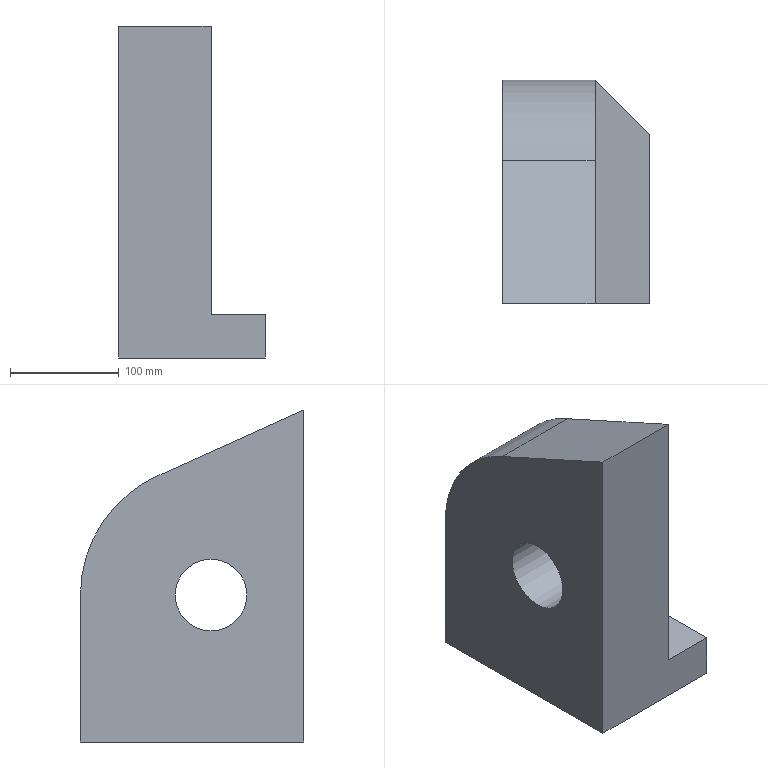Part | NX | features solid 2 | 1 solid | 11 faces | box 135 x 205 x 305 mm | volume 4488992 mm3 | plane 9 | cylinder 2 | commonest cylinder face diameters 66 x1 240 x1
STEP:
#1=CARTESIAN_POINT('',(1415.,1020.,-375.));
#2=VERTEX_POINT('',#1);
#3=CARTESIAN_POINT('',(1415.,1020.,-680.));
#4=VERTEX_POINT('',#3);
#5=CARTESIAN_POINT('',(1415.,1020.,-330.));
#6=DIRECTION('',(0.,0.,-1.));
#7=VECTOR('',#6,1000.);
#8=LINE('',#5,#7);
#9=EDGE_CURVE('',#2,#4,#8,.T.);
#10=ORIENTED_EDGE('',*,*,#9,.T.);
#11=CARTESIAN_POINT('',(1550.,1020.,-680.));
#12=VERTEX_POINT('',#11);
#13=CARTESIAN_POINT('',(1550.,1020.,-680.));
#14=DIRECTION('',(1.,0.,0.));
#15=VECTOR('',#14,1000.);
#16=LINE('',#13,#15);
#17=EDGE_CURVE('',#4,#12,#16,.T.);
#18=ORIENTED_EDGE('',*,*,#17,.T.);
#19=CARTESIAN_POINT('',(1550.,1020.,-640.));
#20=VERTEX_POINT('',#19);
#21=CARTESIAN_POINT('',(1550.,1020.,-575.));
#22=DIRECTION('',(0.,0.,1.));
#23=VECTOR('',#22,1000.);
#24=LINE('',#21,#23);
#25=EDGE_CURVE('',#12,#20,#24,.T.);
#26=ORIENTED_EDGE('',*,*,#25,.T.);
#27=CARTESIAN_POINT('',(1500.,1020.,-640.));
#28=VERTEX_POINT('',#27);
#29=CARTESIAN_POINT('',(-1361.187,1020.,-640.));
#30=DIRECTION('',(1.,0.,0.));
#31=VECTOR('',#30,1000.);
#32=LINE('',#29,#31);
#33=EDGE_CURVE('',#28,#20,#32,.T.);
#34=ORIENTED_EDGE('',*,*,#33,.F.);
#35=CARTESIAN_POINT('',(1500.,1020.,-375.));
#36=VERTEX_POINT('',#35);
#37=CARTESIAN_POINT('',(1500.,1020.,-330.));
#38=DIRECTION('',(0.,0.,-1.));
#39=VECTOR('',#38,1000.);
#40=LINE('',#37,#39);
#41=EDGE_CURVE('',#36,#28,#40,.T.);
#42=ORIENTED_EDGE('',*,*,#41,.F.);
#43=CARTESIAN_POINT('',(1550.,1020.,-375.));
#44=DIRECTION('',(1.,0.,0.));
#45=VECTOR('',#44,1000.);
#46=LINE('',#43,#45);
#47=EDGE_CURVE('',#2,#36,#46,.T.);
#48=ORIENTED_EDGE('',*,*,#47,.F.);
#49=EDGE_LOOP('',(#10,#18,#26,#34,#42,#48));
#50=FACE_BOUND('',#49,.T.);
#51=CARTESIAN_POINT('',(1550.,1020.,-425.));
#52=DIRECTION('',(0.,-1.,0.));
#53=DIRECTION('',(0.,0.,1.));
#54=AXIS2_PLACEMENT_3D('',#51,#52,#53);
#55=PLANE('',#54);
#56=ADVANCED_FACE('',(#50),#55,.T.);
#57=ORIENTED_EDGE('',*,*,#25,.F.);
#58=CARTESIAN_POINT('',(1550.,1175.,-680.));
#59=VERTEX_POINT('',#58);
#60=CARTESIAN_POINT('',(1550.,-830.,-680.));
#61=DIRECTION('',(0.,1.,0.));
#62=VECTOR('',#61,1000.);
#63=LINE('',#60,#62);
#64=EDGE_CURVE('',#12,#59,#63,.T.);
#65=ORIENTED_EDGE('',*,*,#64,.T.);
#66=CARTESIAN_POINT('',(1550.,1175.,-640.));
#67=VERTEX_POINT('',#66);
#68=CARTESIAN_POINT('',(1550.,1175.,-615.));
#69=DIRECTION('',(0.,0.,-1.));
#70=VECTOR('',#69,1000.);
#71=LINE('',#68,#70);
#72=EDGE_CURVE('',#59,#67,#71,.F.);
#73=ORIENTED_EDGE('',*,*,#72,.T.);
#74=CARTESIAN_POINT('',(1550.,-830.,-640.));
#75=DIRECTION('',(0.,-1.,0.));
#76=VECTOR('',#75,1000.);
#77=LINE('',#74,#76);
#78=EDGE_CURVE('',#67,#20,#77,.T.);
#79=ORIENTED_EDGE('',*,*,#78,.T.);
#80=EDGE_LOOP('',(#57,#65,#73,#79));
#81=FACE_BOUND('',#80,.T.);
#82=CARTESIAN_POINT('',(1550.,-830.,-575.));
#83=DIRECTION('',(1.,0.,0.));
#84=DIRECTION('',(0.,0.,1.));
#85=AXIS2_PLACEMENT_3D('',#82,#83,#84);
#86=PLANE('',#85);
#87=ADVANCED_FACE('',(#81),#86,.T.);
#88=ORIENTED_EDGE('',*,*,#33,.T.);
#89=ORIENTED_EDGE('',*,*,#78,.F.);
#90=CARTESIAN_POINT('',(1500.,1225.,-640.));
#91=VERTEX_POINT('',#90);
#92=CARTESIAN_POINT('',(171.907,2553.093,-640.));
#93=DIRECTION('',(0.7071,-0.7071,0.));
#94=VECTOR('',#93,1000.);
#95=LINE('',#92,#94);
#96=EDGE_CURVE('',#67,#91,#95,.F.);
#97=ORIENTED_EDGE('',*,*,#96,.T.);
#98=CARTESIAN_POINT('',(1500.,1230.,-640.));
#99=DIRECTION('',(0.,-1.,0.));
#100=VECTOR('',#99,1000.);
#101=LINE('',#98,#100);
#102=EDGE_CURVE('',#91,#28,#101,.T.);
#103=ORIENTED_EDGE('',*,*,#102,.T.);
#104=EDGE_LOOP('',(#88,#89,#97,#103));
#105=FACE_BOUND('',#104,.T.);
#106=CARTESIAN_POINT('',(-1361.187,1020.,-640.));
#107=DIRECTION('',(0.,0.,-1.));
#108=DIRECTION('',(-1.,0.,0.));
#109=AXIS2_PLACEMENT_3D('',#106,#107,#108);
#110=PLANE('',#109);
#111=ADVANCED_FACE('',(#105),#110,.F.);
#112=CARTESIAN_POINT('',(1500.,1150.971,-434.155));
#113=VERTEX_POINT('',#112);
#114=CARTESIAN_POINT('',(1500.,1177.538,-446.154));
#115=DIRECTION('',(0.,0.9114,-0.4116));
#116=VECTOR('',#115,1000.);
#117=LINE('',#114,#116);
#118=EDGE_CURVE('',#36,#113,#117,.T.);
#119=ORIENTED_EDGE('',*,*,#118,.F.);
#120=ORIENTED_EDGE('',*,*,#41,.T.);
#121=ORIENTED_EDGE('',*,*,#102,.F.);
#122=CARTESIAN_POINT('',(1500.,1225.,-545.));
#123=VERTEX_POINT('',#122);
#124=CARTESIAN_POINT('',(1500.,1225.,-560.));
#125=DIRECTION('',(0.,0.,-1.));
#126=VECTOR('',#125,1000.);
#127=LINE('',#124,#126);
#128=EDGE_CURVE('',#123,#91,#127,.T.);
#129=ORIENTED_EDGE('',*,*,#128,.F.);
#130=CARTESIAN_POINT('',(1500.,1105.,-545.));
#131=DIRECTION('',(-1.,0.,0.));
#132=DIRECTION('',(0.,0.,-1.));
#133=AXIS2_PLACEMENT_3D('',#130,#131,#132);
#134=CIRCLE('',#133,120.);
#135=EDGE_CURVE('',#123,#113,#134,.F.);
#136=ORIENTED_EDGE('',*,*,#135,.T.);
#137=EDGE_LOOP('',(#119,#120,#121,#129,#136));
#138=FACE_BOUND('',#137,.T.);
#139=CARTESIAN_POINT('',(1500.,1105.,-578.));
#140=VERTEX_POINT('',#139);
#141=CARTESIAN_POINT('',(1500.,1105.,-545.));
#142=DIRECTION('',(-1.,0.,0.));
#143=DIRECTION('',(0.,0.,-1.));
#144=AXIS2_PLACEMENT_3D('',#141,#142,#143);
#145=CIRCLE('',#144,33.);
#146=EDGE_CURVE('',#140,#140,#145,.T.);
#147=ORIENTED_EDGE('',*,*,#146,.T.);
#148=EDGE_LOOP('',(#147));
#149=FACE_BOUND('',#148,.T.);
#150=CARTESIAN_POINT('',(1500.,1230.,-330.));
#151=DIRECTION('',(1.,0.,0.));
#152=DIRECTION('',(0.,1.,0.));
#153=AXIS2_PLACEMENT_3D('',#150,#151,#152);
#154=PLANE('',#153);
#155=ADVANCED_FACE('',(#138,#149),#154,.T.);
#156=ORIENTED_EDGE('',*,*,#146,.F.);
#157=EDGE_LOOP('',(#156));
#158=FACE_BOUND('',#157,.T.);
#159=CARTESIAN_POINT('',(1415.,1105.,-578.));
#160=VERTEX_POINT('',#159);
#161=CARTESIAN_POINT('',(1415.,1105.,-545.));
#162=DIRECTION('',(-1.,0.,0.));
#163=DIRECTION('',(0.,0.,-1.));
#164=AXIS2_PLACEMENT_3D('',#161,#162,#163);
#165=CIRCLE('',#164,33.);
#166=EDGE_CURVE('',#160,#160,#165,.F.);
#167=ORIENTED_EDGE('',*,*,#166,.F.);
#168=EDGE_LOOP('',(#167));
#169=FACE_BOUND('',#168,.T.);
#170=CARTESIAN_POINT('',(1535.,1105.,-545.));
#171=DIRECTION('',(-1.,0.,0.));
#172=DIRECTION('',(0.,0.,-1.));
#173=AXIS2_PLACEMENT_3D('',#170,#171,#172);
#174=CYLINDRICAL_SURFACE('',#173,33.);
#175=ADVANCED_FACE('',(#158,#169),#174,.F.);
#176=CARTESIAN_POINT('',(1415.,1150.971,-434.155));
#177=VERTEX_POINT('',#176);
#178=CARTESIAN_POINT('',(1215.,1150.971,-434.155));
#179=DIRECTION('',(1.,0.,0.));
#180=VECTOR('',#179,1000.);
#181=LINE('',#178,#180);
#182=EDGE_CURVE('',#113,#177,#181,.F.);
#183=ORIENTED_EDGE('',*,*,#182,.F.);
#184=ORIENTED_EDGE('',*,*,#135,.F.);
#185=CARTESIAN_POINT('',(1415.,1225.,-545.));
#186=VERTEX_POINT('',#185);
#187=CARTESIAN_POINT('',(1215.,1225.,-545.));
#188=DIRECTION('',(-1.,0.,0.));
#189=VECTOR('',#188,1000.);
#190=LINE('',#187,#189);
#191=EDGE_CURVE('',#186,#123,#190,.F.);
#192=ORIENTED_EDGE('',*,*,#191,.F.);
#193=CARTESIAN_POINT('',(1415.,1105.,-545.));
#194=DIRECTION('',(-1.,0.,0.));
#195=DIRECTION('',(0.,0.,-1.));
#196=AXIS2_PLACEMENT_3D('',#193,#194,#195);
#197=CIRCLE('',#196,120.);
#198=EDGE_CURVE('',#177,#186,#197,.T.);
#199=ORIENTED_EDGE('',*,*,#198,.F.);
#200=EDGE_LOOP('',(#183,#184,#192,#199));
#201=FACE_BOUND('',#200,.T.);
#202=CARTESIAN_POINT('',(1215.,1105.,-545.));
#203=DIRECTION('',(1.,0.,0.));
#204=DIRECTION('',(0.,0.,-1.));
#205=AXIS2_PLACEMENT_3D('',#202,#203,#204);
#206=CYLINDRICAL_SURFACE('',#205,120.);
#207=ADVANCED_FACE('',(#201),#206,.T.);
#208=CARTESIAN_POINT('',(1500.,1225.,-680.));
#209=VERTEX_POINT('',#208);
#210=CARTESIAN_POINT('',(1415.,1225.,-680.));
#211=VERTEX_POINT('',#210);
#212=CARTESIAN_POINT('',(1215.,1225.,-680.));
#213=DIRECTION('',(-1.,0.,0.));
#214=VECTOR('',#213,1000.);
#215=LINE('',#212,#214);
#216=EDGE_CURVE('',#209,#211,#215,.T.);
#217=ORIENTED_EDGE('',*,*,#216,.T.);
#218=CARTESIAN_POINT('',(1415.,1225.,-330.));
#219=DIRECTION('',(0.,0.,1.));
#220=VECTOR('',#219,1000.);
#221=LINE('',#218,#220);
#222=EDGE_CURVE('',#211,#186,#221,.T.);
#223=ORIENTED_EDGE('',*,*,#222,.T.);
#224=ORIENTED_EDGE('',*,*,#191,.T.);
#225=ORIENTED_EDGE('',*,*,#128,.T.);
#226=CARTESIAN_POINT('',(1500.,1225.,-655.));
#227=DIRECTION('',(0.,0.,-1.));
#228=VECTOR('',#227,1000.);
#229=LINE('',#226,#228);
#230=EDGE_CURVE('',#91,#209,#229,.T.);
#231=ORIENTED_EDGE('',*,*,#230,.T.);
#232=EDGE_LOOP('',(#217,#223,#224,#225,#231));
#233=FACE_BOUND('',#232,.T.);
#234=CARTESIAN_POINT('',(1215.,1225.,-560.));
#235=DIRECTION('',(0.,1.,0.));
#236=DIRECTION('',(-1.,0.,0.));
#237=AXIS2_PLACEMENT_3D('',#234,#235,#236);
#238=PLANE('',#237);
#239=ADVANCED_FACE('',(#233),#238,.T.);
#240=ORIENTED_EDGE('',*,*,#9,.F.);
#241=CARTESIAN_POINT('',(1415.,1038.757,-383.472));
#242=DIRECTION('',(0.,0.9114,-0.4116));
#243=VECTOR('',#242,1000.);
#244=LINE('',#241,#243);
#245=EDGE_CURVE('',#2,#177,#244,.T.);
#246=ORIENTED_EDGE('',*,*,#245,.T.);
#247=ORIENTED_EDGE('',*,*,#198,.T.);
#248=ORIENTED_EDGE('',*,*,#222,.F.);
#249=CARTESIAN_POINT('',(1415.,1230.,-680.));
#250=DIRECTION('',(0.,1.,0.));
#251=VECTOR('',#250,1000.);
#252=LINE('',#249,#251);
#253=EDGE_CURVE('',#4,#211,#252,.T.);
#254=ORIENTED_EDGE('',*,*,#253,.F.);
#255=EDGE_LOOP('',(#240,#246,#247,#248,#254));
#256=FACE_BOUND('',#255,.T.);
#257=ORIENTED_EDGE('',*,*,#166,.T.);
#258=EDGE_LOOP('',(#257));
#259=FACE_BOUND('',#258,.T.);
#260=CARTESIAN_POINT('',(1415.,1230.,-330.));
#261=DIRECTION('',(1.,0.,0.));
#262=DIRECTION('',(0.,1.,0.));
#263=AXIS2_PLACEMENT_3D('',#260,#261,#262);
#264=PLANE('',#263);
#265=ADVANCED_FACE('',(#256,#259),#264,.F.);
#266=CARTESIAN_POINT('',(1550.,1175.,-680.));
#267=DIRECTION('',(0.7071,-0.7071,0.));
#268=VECTOR('',#267,1000.);
#269=LINE('',#266,#268);
#270=EDGE_CURVE('',#59,#209,#269,.F.);
#271=ORIENTED_EDGE('',*,*,#270,.T.);
#272=ORIENTED_EDGE('',*,*,#230,.F.);
#273=ORIENTED_EDGE('',*,*,#96,.F.);
#274=ORIENTED_EDGE('',*,*,#72,.F.);
#275=EDGE_LOOP('',(#271,#272,#273,#274));
#276=FACE_BOUND('',#275,.T.);
#277=CARTESIAN_POINT('',(1550.,1175.,-575.));
#278=DIRECTION('',(-0.7071,-0.7071,0.));
#279=DIRECTION('',(0.7071,-0.7071,0.));
#280=AXIS2_PLACEMENT_3D('',#277,#278,#279);
#281=PLANE('',#280);
#282=ADVANCED_FACE('',(#276),#281,.F.);
#283=ORIENTED_EDGE('',*,*,#64,.F.);
#284=ORIENTED_EDGE('',*,*,#17,.F.);
#285=ORIENTED_EDGE('',*,*,#253,.T.);
#286=ORIENTED_EDGE('',*,*,#216,.F.);
#287=ORIENTED_EDGE('',*,*,#270,.F.);
#288=EDGE_LOOP('',(#283,#284,#285,#286,#287));
#289=FACE_BOUND('',#288,.T.);
#290=CARTESIAN_POINT('',(80.,-155.,-680.));
#291=DIRECTION('',(0.,0.,1.));
#292=DIRECTION('',(-1.,0.,0.));
#293=AXIS2_PLACEMENT_3D('',#290,#291,#292);
#294=PLANE('',#293);
#295=ADVANCED_FACE('',(#289),#294,.F.);
#296=ORIENTED_EDGE('',*,*,#118,.T.);
#297=ORIENTED_EDGE('',*,*,#182,.T.);
#298=ORIENTED_EDGE('',*,*,#245,.F.);
#299=ORIENTED_EDGE('',*,*,#47,.T.);
#300=EDGE_LOOP('',(#296,#297,#298,#299));
#301=FACE_BOUND('',#300,.T.);
#302=CARTESIAN_POINT('',(1500.,1020.,-375.));
#303=DIRECTION('',(0.,0.4116,0.9114));
#304=DIRECTION('',(0.,0.9114,-0.4116));
#305=AXIS2_PLACEMENT_3D('',#302,#303,#304);
#306=PLANE('',#305);
#307=ADVANCED_FACE('',(#301),#306,.T.);
#308=CLOSED_SHELL('',(#56,#87,#111,#155,#175,#207,#239,#265,#282,#295,#307));
#309=MANIFOLD_SOLID_BREP('',#308);
#310=(LENGTH_UNIT()NAMED_UNIT(*)SI_UNIT(.MILLI.,.METRE.));
#311=UNCERTAINTY_MEASURE_WITH_UNIT(LENGTH_MEASURE(0.00001),#310,'','');
#312=(NAMED_UNIT(*)PLANE_ANGLE_UNIT()SI_UNIT($,.RADIAN.));
#313=(NAMED_UNIT(*)SI_UNIT($,.STERADIAN.)SOLID_ANGLE_UNIT());
#314=(GEOMETRIC_REPRESENTATION_CONTEXT(3)GLOBAL_UNCERTAINTY_ASSIGNED_CONTEXT((#311))GLOBAL_UNIT_ASSIGNED_CONTEXT((#310,#312,#313))REPRESENTATION_CONTEXT('',''));
#315=ADVANCED_BREP_SHAPE_REPRESENTATION('',(#309),#314);